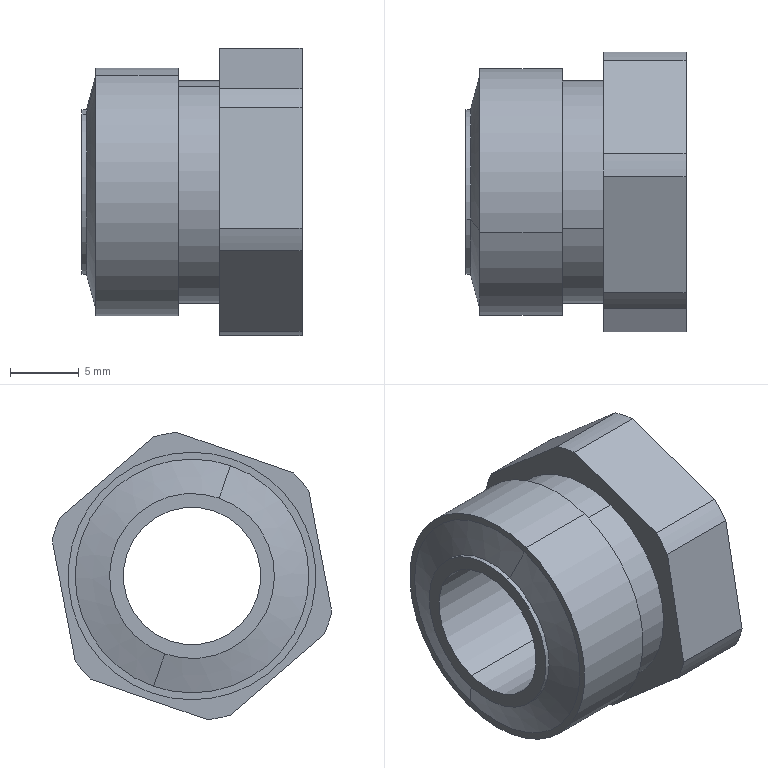Part | SolidWorks | features BaseBody 1 | 1 solid | 30 faces | box 16 x 20.336 x 20.886 mm | volume 2470 mm3 | cylinder 16 | plane 12 | cone 2 | commonest cylinder face diameters 21 x6 10 x2 12 x2 16 x2 16.2 x2 18 x2
STEP:
#1=CARTESIAN_POINT('',(0.03712,-55.457,-220.271));
#2=VERTEX_POINT('',#1);
#3=CARTESIAN_POINT('',(0.03712,-58.751,-210.829));
#4=VERTEX_POINT('',#3);
#5=CARTESIAN_POINT('',(0.03712,-57.104,-215.55));
#6=DIRECTION('',(-1.,0.,0.));
#7=DIRECTION('',(0.,0.3294,-0.9442));
#8=AXIS2_PLACEMENT_3D('',#5,#6,#7);
#9=CIRCLE('',#8,5.);
#10=EDGE_CURVE('',#2,#4,#9,.T.);
#11=ORIENTED_EDGE('',*,*,#10,.F.);
#12=CARTESIAN_POINT('',(-12.463,-55.457,-220.271));
#13=VERTEX_POINT('',#12);
#14=CARTESIAN_POINT('',(3.537,-55.457,-220.271));
#15=DIRECTION('',(-1.,0.,0.));
#16=VECTOR('',#15,1000.);
#17=LINE('',#14,#16);
#18=EDGE_CURVE('',#2,#13,#17,.T.);
#19=ORIENTED_EDGE('',*,*,#18,.T.);
#20=CARTESIAN_POINT('',(-12.463,-58.751,-210.829));
#21=VERTEX_POINT('',#20);
#22=CARTESIAN_POINT('',(-12.463,-57.104,-215.55));
#23=DIRECTION('',(-1.,0.,0.));
#24=DIRECTION('',(0.,-0.3294,0.9442));
#25=AXIS2_PLACEMENT_3D('',#22,#23,#24);
#26=CIRCLE('',#25,5.);
#27=EDGE_CURVE('',#13,#21,#26,.T.);
#28=ORIENTED_EDGE('',*,*,#27,.T.);
#29=CARTESIAN_POINT('',(3.537,-58.751,-210.829));
#30=DIRECTION('',(-1.,0.,0.));
#31=VECTOR('',#30,1000.);
#32=LINE('',#29,#31);
#33=EDGE_CURVE('',#4,#21,#32,.T.);
#34=ORIENTED_EDGE('',*,*,#33,.F.);
#35=EDGE_LOOP('',(#11,#19,#28,#34));
#36=FACE_OUTER_BOUND('',#35,.T.);
#37=CARTESIAN_POINT('',(3.537,-57.104,-215.55));
#38=DIRECTION('',(-1.,0.,0.));
#39=DIRECTION('',(0.,-0.3294,0.9442));
#40=AXIS2_PLACEMENT_3D('',#37,#38,#39);
#41=CYLINDRICAL_SURFACE('',#40,5.);
#42=ADVANCED_FACE('',(#36),#41,.F.);
#43=CARTESIAN_POINT('',(-5.463,-59.772,-207.902));
#44=VERTEX_POINT('',#43);
#45=CARTESIAN_POINT('',(-5.463,-54.435,-223.198));
#46=VERTEX_POINT('',#45);
#47=CARTESIAN_POINT('',(-5.463,-57.104,-215.55));
#48=DIRECTION('',(-1.,0.,0.));
#49=DIRECTION('',(0.,-0.3294,0.9442));
#50=AXIS2_PLACEMENT_3D('',#47,#48,#49);
#51=CIRCLE('',#50,8.1);
#52=EDGE_CURVE('',#44,#46,#51,.T.);
#53=ORIENTED_EDGE('',*,*,#52,.F.);
#54=CARTESIAN_POINT('',(-2.463,-59.772,-207.902));
#55=VERTEX_POINT('',#54);
#56=CARTESIAN_POINT('',(-5.463,-59.772,-207.902));
#57=DIRECTION('',(1.,0.,0.));
#58=VECTOR('',#57,1000.);
#59=LINE('',#56,#58);
#60=EDGE_CURVE('',#44,#55,#59,.T.);
#61=ORIENTED_EDGE('',*,*,#60,.T.);
#62=CARTESIAN_POINT('',(-2.463,-54.435,-223.198));
#63=VERTEX_POINT('',#62);
#64=CARTESIAN_POINT('',(-2.463,-57.104,-215.55));
#65=DIRECTION('',(-1.,0.,0.));
#66=DIRECTION('',(0.,-0.3294,0.9442));
#67=AXIS2_PLACEMENT_3D('',#64,#65,#66);
#68=CIRCLE('',#67,8.1);
#69=EDGE_CURVE('',#55,#63,#68,.T.);
#70=ORIENTED_EDGE('',*,*,#69,.T.);
#71=CARTESIAN_POINT('',(-5.463,-54.435,-223.198));
#72=DIRECTION('',(1.,0.,0.));
#73=VECTOR('',#72,1000.);
#74=LINE('',#71,#73);
#75=EDGE_CURVE('',#46,#63,#74,.T.);
#76=ORIENTED_EDGE('',*,*,#75,.F.);
#77=EDGE_LOOP('',(#53,#61,#70,#76));
#78=FACE_OUTER_BOUND('',#77,.T.);
#79=CARTESIAN_POINT('',(-5.463,-57.104,-215.55));
#80=DIRECTION('',(1.,0.,0.));
#81=DIRECTION('',(0.,0.3294,-0.9442));
#82=AXIS2_PLACEMENT_3D('',#79,#80,#81);
#83=CYLINDRICAL_SURFACE('',#82,8.1);
#84=ADVANCED_FACE('',(#78),#83,.T.);
#85=CARTESIAN_POINT('',(-11.463,-60.069,-207.052));
#86=VERTEX_POINT('',#85);
#87=CARTESIAN_POINT('',(-11.463,-54.139,-224.048));
#88=VERTEX_POINT('',#87);
#89=CARTESIAN_POINT('',(-11.463,-57.104,-215.55));
#90=DIRECTION('',(-1.,0.,0.));
#91=DIRECTION('',(0.,-0.3294,0.9442));
#92=AXIS2_PLACEMENT_3D('',#89,#90,#91);
#93=CIRCLE('',#92,9.);
#94=EDGE_CURVE('',#86,#88,#93,.T.);
#95=ORIENTED_EDGE('',*,*,#94,.F.);
#96=CARTESIAN_POINT('',(-5.463,-60.069,-207.052));
#97=VERTEX_POINT('',#96);
#98=CARTESIAN_POINT('',(-11.463,-60.069,-207.052));
#99=DIRECTION('',(1.,0.,0.));
#100=VECTOR('',#99,1000.);
#101=LINE('',#98,#100);
#102=EDGE_CURVE('',#86,#97,#101,.T.);
#103=ORIENTED_EDGE('',*,*,#102,.T.);
#104=CARTESIAN_POINT('',(-5.463,-54.139,-224.048));
#105=VERTEX_POINT('',#104);
#106=CARTESIAN_POINT('',(-5.463,-57.104,-215.55));
#107=DIRECTION('',(-1.,0.,0.));
#108=DIRECTION('',(0.,-0.3294,0.9442));
#109=AXIS2_PLACEMENT_3D('',#106,#107,#108);
#110=CIRCLE('',#109,9.);
#111=EDGE_CURVE('',#97,#105,#110,.T.);
#112=ORIENTED_EDGE('',*,*,#111,.T.);
#113=CARTESIAN_POINT('',(-11.463,-54.139,-224.048));
#114=DIRECTION('',(1.,0.,0.));
#115=VECTOR('',#114,1000.);
#116=LINE('',#113,#115);
#117=EDGE_CURVE('',#88,#105,#116,.T.);
#118=ORIENTED_EDGE('',*,*,#117,.F.);
#119=EDGE_LOOP('',(#95,#103,#112,#118));
#120=FACE_OUTER_BOUND('',#119,.T.);
#121=CARTESIAN_POINT('',(-11.463,-57.104,-215.55));
#122=DIRECTION('',(1.,0.,0.));
#123=DIRECTION('',(0.,0.3294,-0.9442));
#124=AXIS2_PLACEMENT_3D('',#121,#122,#123);
#125=CYLINDRICAL_SURFACE('',#124,9.);
#126=ADVANCED_FACE('',(#120),#125,.T.);
#127=CARTESIAN_POINT('',(-12.463,-59.08,-209.885));
#128=VERTEX_POINT('',#127);
#129=CARTESIAN_POINT('',(-12.463,-55.127,-221.215));
#130=VERTEX_POINT('',#129);
#131=CARTESIAN_POINT('',(-12.463,-57.104,-215.55));
#132=DIRECTION('',(-1.,0.,0.));
#133=DIRECTION('',(0.,-0.3294,0.9442));
#134=AXIS2_PLACEMENT_3D('',#131,#132,#133);
#135=CIRCLE('',#134,6.);
#136=EDGE_CURVE('',#128,#130,#135,.T.);
#137=ORIENTED_EDGE('',*,*,#136,.F.);
#138=CARTESIAN_POINT('',(-12.133,-59.08,-209.885));
#139=VERTEX_POINT('',#138);
#140=CARTESIAN_POINT('',(-12.463,-59.08,-209.885));
#141=DIRECTION('',(1.,0.,0.));
#142=VECTOR('',#141,1000.);
#143=LINE('',#140,#142);
#144=EDGE_CURVE('',#128,#139,#143,.T.);
#145=ORIENTED_EDGE('',*,*,#144,.T.);
#146=CARTESIAN_POINT('',(-12.133,-55.127,-221.215));
#147=VERTEX_POINT('',#146);
#148=CARTESIAN_POINT('',(-12.133,-57.104,-215.55));
#149=DIRECTION('',(-1.,0.,0.));
#150=DIRECTION('',(0.,-0.3294,0.9442));
#151=AXIS2_PLACEMENT_3D('',#148,#149,#150);
#152=CIRCLE('',#151,6.);
#153=EDGE_CURVE('',#139,#147,#152,.T.);
#154=ORIENTED_EDGE('',*,*,#153,.T.);
#155=CARTESIAN_POINT('',(-12.463,-55.127,-221.215));
#156=DIRECTION('',(1.,0.,0.));
#157=VECTOR('',#156,1000.);
#158=LINE('',#155,#157);
#159=EDGE_CURVE('',#130,#147,#158,.T.);
#160=ORIENTED_EDGE('',*,*,#159,.F.);
#161=EDGE_LOOP('',(#137,#145,#154,#160));
#162=FACE_OUTER_BOUND('',#161,.T.);
#163=CARTESIAN_POINT('',(-12.463,-57.104,-215.55));
#164=DIRECTION('',(1.,0.,0.));
#165=DIRECTION('',(0.,0.3294,-0.9442));
#166=AXIS2_PLACEMENT_3D('',#163,#164,#165);
#167=CYLINDRICAL_SURFACE('',#166,6.);
#168=ADVANCED_FACE('',(#162),#167,.T.);
#169=ORIENTED_EDGE('',*,*,#153,.F.);
#170=CARTESIAN_POINT('',(-11.463,-59.904,-207.525));
#171=VERTEX_POINT('',#170);
#172=CARTESIAN_POINT('',(-12.133,-59.08,-209.885));
#173=DIRECTION('',(0.2588,-0.3182,0.912));
#174=VECTOR('',#173,1000.);
#175=LINE('',#172,#174);
#176=EDGE_CURVE('',#139,#171,#175,.T.);
#177=ORIENTED_EDGE('',*,*,#176,.T.);
#178=CARTESIAN_POINT('',(-11.463,-54.303,-223.575));
#179=VERTEX_POINT('',#178);
#180=CARTESIAN_POINT('',(-11.463,-57.104,-215.55));
#181=DIRECTION('',(1.,0.,0.));
#182=DIRECTION('',(0.,-0.3294,0.9442));
#183=AXIS2_PLACEMENT_3D('',#180,#181,#182);
#184=CIRCLE('',#183,8.5);
#185=EDGE_CURVE('',#179,#171,#184,.T.);
#186=ORIENTED_EDGE('',*,*,#185,.F.);
#187=CARTESIAN_POINT('',(-12.133,-55.127,-221.215));
#188=DIRECTION('',(0.2588,0.3182,-0.912));
#189=VECTOR('',#188,1000.);
#190=LINE('',#187,#189);
#191=EDGE_CURVE('',#147,#179,#190,.T.);
#192=ORIENTED_EDGE('',*,*,#191,.F.);
#193=EDGE_LOOP('',(#169,#177,#186,#192));
#194=FACE_OUTER_BOUND('',#193,.T.);
#195=CARTESIAN_POINT('',(-12.133,-57.104,-215.55));
#196=DIRECTION('',(1.,0.,0.));
#197=DIRECTION('',(0.,0.3294,-0.9442));
#198=AXIS2_PLACEMENT_3D('',#195,#196,#197);
#199=CONICAL_SURFACE('',#198,6.,1.309);
#200=ADVANCED_FACE('',(#194),#199,.T.);
#201=CARTESIAN_POINT('',(0.03712,-59.739,-207.997));
#202=VERTEX_POINT('',#201);
#203=CARTESIAN_POINT('',(0.03712,-54.468,-223.103));
#204=VERTEX_POINT('',#203);
#205=CARTESIAN_POINT('',(0.03712,-57.104,-215.55));
#206=DIRECTION('',(1.,0.,0.));
#207=DIRECTION('',(0.,0.3294,-0.9442));
#208=AXIS2_PLACEMENT_3D('',#205,#206,#207);
#209=CIRCLE('',#208,8.);
#210=EDGE_CURVE('',#202,#204,#209,.T.);
#211=ORIENTED_EDGE('',*,*,#210,.F.);
#212=CARTESIAN_POINT('',(3.537,-59.739,-207.997));
#213=VERTEX_POINT('',#212);
#214=CARTESIAN_POINT('',(0.03712,-59.739,-207.997));
#215=DIRECTION('',(1.,0.,0.));
#216=VECTOR('',#215,1000.);
#217=LINE('',#214,#216);
#218=EDGE_CURVE('',#202,#213,#217,.T.);
#219=ORIENTED_EDGE('',*,*,#218,.T.);
#220=CARTESIAN_POINT('',(3.537,-54.468,-223.103));
#221=VERTEX_POINT('',#220);
#222=CARTESIAN_POINT('',(3.537,-57.104,-215.55));
#223=DIRECTION('',(1.,0.,0.));
#224=DIRECTION('',(0.,0.3294,-0.9442));
#225=AXIS2_PLACEMENT_3D('',#222,#223,#224);
#226=CIRCLE('',#225,8.);
#227=EDGE_CURVE('',#213,#221,#226,.T.);
#228=ORIENTED_EDGE('',*,*,#227,.T.);
#229=CARTESIAN_POINT('',(0.03712,-54.468,-223.103));
#230=DIRECTION('',(1.,0.,0.));
#231=VECTOR('',#230,1000.);
#232=LINE('',#229,#231);
#233=EDGE_CURVE('',#204,#221,#232,.T.);
#234=ORIENTED_EDGE('',*,*,#233,.F.);
#235=EDGE_LOOP('',(#211,#219,#228,#234));
#236=FACE_OUTER_BOUND('',#235,.T.);
#237=CARTESIAN_POINT('',(0.03712,-57.104,-215.55));
#238=DIRECTION('',(1.,0.,0.));
#239=DIRECTION('',(0.,0.3294,-0.9442));
#240=AXIS2_PLACEMENT_3D('',#237,#238,#239);
#241=CYLINDRICAL_SURFACE('',#240,8.);
#242=ADVANCED_FACE('',(#236),#241,.F.);
#243=CARTESIAN_POINT('',(-2.463,-65.601,-209.382));
#244=VERTEX_POINT('',#243);
#245=CARTESIAN_POINT('',(3.537,-65.601,-209.382));
#246=VERTEX_POINT('',#245);
#247=CARTESIAN_POINT('',(-2.463,-65.601,-209.382));
#248=DIRECTION('',(1.,0.,0.));
#249=VECTOR('',#248,1000.);
#250=LINE('',#247,#249);
#251=EDGE_CURVE('',#244,#246,#250,.T.);
#252=ORIENTED_EDGE('',*,*,#251,.F.);
#253=CARTESIAN_POINT('',(-2.463,-67.272,-218.169));
#254=VERTEX_POINT('',#253);
#255=CARTESIAN_POINT('',(-2.463,-66.437,-213.776));
#256=DIRECTION('',(0.,-0.1868,-0.9824));
#257=VECTOR('',#256,1000.);
#258=LINE('',#255,#257);
#259=EDGE_CURVE('',#244,#254,#258,.T.);
#260=ORIENTED_EDGE('',*,*,#259,.T.);
#261=CARTESIAN_POINT('',(3.537,-67.272,-218.169));
#262=VERTEX_POINT('',#261);
#263=CARTESIAN_POINT('',(-2.463,-67.272,-218.169));
#264=DIRECTION('',(-1.,0.,0.));
#265=VECTOR('',#264,1000.);
#266=LINE('',#263,#265);
#267=EDGE_CURVE('',#262,#254,#266,.T.);
#268=ORIENTED_EDGE('',*,*,#267,.F.);
#269=CARTESIAN_POINT('',(3.537,-67.461,-219.164));
#270=DIRECTION('',(0.,0.1868,0.9824));
#271=VECTOR('',#270,1000.);
#272=LINE('',#269,#271);
#273=EDGE_CURVE('',#262,#246,#272,.T.);
#274=ORIENTED_EDGE('',*,*,#273,.T.);
#275=EDGE_LOOP('',(#252,#260,#268,#274));
#276=FACE_OUTER_BOUND('',#275,.T.);
#277=CARTESIAN_POINT('',(-12.463,-67.461,-219.164));
#278=DIRECTION('',(0.,0.9824,-0.1868));
#279=DIRECTION('',(-1.,0.,0.));
#280=AXIS2_PLACEMENT_3D('',#277,#278,#279);
#281=PLANE('',#280);
#282=ADVANCED_FACE('',(#276),#281,.F.);
#283=CARTESIAN_POINT('',(-2.463,-64.456,-208.054));
#284=VERTEX_POINT('',#283);
#285=CARTESIAN_POINT('',(-2.463,-56.011,-205.107));
#286=VERTEX_POINT('',#285);
#287=CARTESIAN_POINT('',(-2.463,-60.234,-206.58));
#288=DIRECTION('',(0.,0.9442,0.3294));
#289=VECTOR('',#288,1000.);
#290=LINE('',#287,#289);
#291=EDGE_CURVE('',#284,#286,#290,.T.);
#292=ORIENTED_EDGE('',*,*,#291,.F.);
#293=CARTESIAN_POINT('',(3.537,-64.456,-208.054));
#294=VERTEX_POINT('',#293);
#295=CARTESIAN_POINT('',(-2.463,-64.456,-208.054));
#296=DIRECTION('',(1.,0.,0.));
#297=VECTOR('',#296,1000.);
#298=LINE('',#295,#297);
#299=EDGE_CURVE('',#284,#294,#298,.T.);
#300=ORIENTED_EDGE('',*,*,#299,.T.);
#301=CARTESIAN_POINT('',(3.537,-56.011,-205.107));
#302=VERTEX_POINT('',#301);
#303=CARTESIAN_POINT('',(3.537,-55.055,-204.773));
#304=DIRECTION('',(0.,-0.9442,-0.3294));
#305=VECTOR('',#304,1000.);
#306=LINE('',#303,#305);
#307=EDGE_CURVE('',#302,#294,#306,.T.);
#308=ORIENTED_EDGE('',*,*,#307,.F.);
#309=CARTESIAN_POINT('',(-2.463,-56.011,-205.107));
#310=DIRECTION('',(-1.,0.,0.));
#311=VECTOR('',#310,1000.);
#312=LINE('',#309,#311);
#313=EDGE_CURVE('',#302,#286,#312,.T.);
#314=ORIENTED_EDGE('',*,*,#313,.T.);
#315=EDGE_LOOP('',(#292,#300,#308,#314));
#316=FACE_OUTER_BOUND('',#315,.T.);
#317=CARTESIAN_POINT('',(-12.463,-55.055,-204.773));
#318=DIRECTION('',(0.,-0.3294,0.9442));
#319=DIRECTION('',(-1.,0.,0.));
#320=AXIS2_PLACEMENT_3D('',#317,#318,#319);
#321=PLANE('',#320);
#322=ADVANCED_FACE('',(#316),#321,.T.);
#323=CARTESIAN_POINT('',(-2.463,-54.288,-205.435));
#324=VERTEX_POINT('',#323);
#325=CARTESIAN_POINT('',(-2.463,-47.514,-211.275));
#326=VERTEX_POINT('',#325);
#327=CARTESIAN_POINT('',(-2.463,-50.901,-208.355));
#328=DIRECTION('',(0.,0.7574,-0.653));
#329=VECTOR('',#328,1000.);
#330=LINE('',#327,#329);
#331=EDGE_CURVE('',#324,#326,#330,.T.);
#332=ORIENTED_EDGE('',*,*,#331,.F.);
#333=CARTESIAN_POINT('',(3.537,-54.288,-205.435));
#334=VERTEX_POINT('',#333);
#335=CARTESIAN_POINT('',(-2.463,-54.288,-205.435));
#336=DIRECTION('',(1.,0.,0.));
#337=VECTOR('',#336,1000.);
#338=LINE('',#335,#337);
#339=EDGE_CURVE('',#324,#334,#338,.T.);
#340=ORIENTED_EDGE('',*,*,#339,.T.);
#341=CARTESIAN_POINT('',(3.537,-47.514,-211.275));
#342=VERTEX_POINT('',#341);
#343=CARTESIAN_POINT('',(3.537,-46.747,-211.936));
#344=DIRECTION('',(0.,-0.7574,0.653));
#345=VECTOR('',#344,1000.);
#346=LINE('',#343,#345);
#347=EDGE_CURVE('',#342,#334,#346,.T.);
#348=ORIENTED_EDGE('',*,*,#347,.F.);
#349=CARTESIAN_POINT('',(-2.463,-47.514,-211.275));
#350=DIRECTION('',(-1.,0.,0.));
#351=VECTOR('',#350,1000.);
#352=LINE('',#349,#351);
#353=EDGE_CURVE('',#342,#326,#352,.T.);
#354=ORIENTED_EDGE('',*,*,#353,.T.);
#355=EDGE_LOOP('',(#332,#340,#348,#354));
#356=FACE_OUTER_BOUND('',#355,.T.);
#357=CARTESIAN_POINT('',(-12.463,-46.747,-211.936));
#358=DIRECTION('',(0.,0.653,0.7574));
#359=DIRECTION('',(1.,0.,0.));
#360=AXIS2_PLACEMENT_3D('',#357,#358,#359);
#361=PLANE('',#360);
#362=ADVANCED_FACE('',(#356),#361,.T.);
#363=CARTESIAN_POINT('',(-2.463,-48.606,-221.718));
#364=VERTEX_POINT('',#363);
#365=CARTESIAN_POINT('',(3.537,-48.606,-221.718));
#366=VERTEX_POINT('',#365);
#367=CARTESIAN_POINT('',(-2.463,-48.606,-221.718));
#368=DIRECTION('',(1.,0.,0.));
#369=VECTOR('',#368,1000.);
#370=LINE('',#367,#369);
#371=EDGE_CURVE('',#364,#366,#370,.T.);
#372=ORIENTED_EDGE('',*,*,#371,.F.);
#373=CARTESIAN_POINT('',(-2.463,-46.936,-212.931));
#374=VERTEX_POINT('',#373);
#375=CARTESIAN_POINT('',(-2.463,-47.771,-217.324));
#376=DIRECTION('',(0.,0.1868,0.9824));
#377=VECTOR('',#376,1000.);
#378=LINE('',#375,#377);
#379=EDGE_CURVE('',#364,#374,#378,.T.);
#380=ORIENTED_EDGE('',*,*,#379,.T.);
#381=CARTESIAN_POINT('',(3.537,-46.936,-212.931));
#382=VERTEX_POINT('',#381);
#383=CARTESIAN_POINT('',(-2.463,-46.936,-212.931));
#384=DIRECTION('',(-1.,0.,0.));
#385=VECTOR('',#384,1000.);
#386=LINE('',#383,#385);
#387=EDGE_CURVE('',#382,#374,#386,.T.);
#388=ORIENTED_EDGE('',*,*,#387,.F.);
#389=CARTESIAN_POINT('',(3.537,-46.747,-211.936));
#390=DIRECTION('',(0.,-0.1868,-0.9824));
#391=VECTOR('',#390,1000.);
#392=LINE('',#389,#391);
#393=EDGE_CURVE('',#382,#366,#392,.T.);
#394=ORIENTED_EDGE('',*,*,#393,.T.);
#395=EDGE_LOOP('',(#372,#380,#388,#394));
#396=FACE_OUTER_BOUND('',#395,.T.);
#397=CARTESIAN_POINT('',(-12.463,-46.747,-211.936));
#398=DIRECTION('',(0.,-0.9824,0.1868));
#399=DIRECTION('',(-1.,0.,0.));
#400=AXIS2_PLACEMENT_3D('',#397,#398,#399);
#401=PLANE('',#400);
#402=ADVANCED_FACE('',(#396),#401,.F.);
#403=CARTESIAN_POINT('',(-2.463,-58.196,-225.993));
#404=VERTEX_POINT('',#403);
#405=CARTESIAN_POINT('',(3.537,-58.196,-225.993));
#406=VERTEX_POINT('',#405);
#407=CARTESIAN_POINT('',(-2.463,-58.196,-225.993));
#408=DIRECTION('',(1.,0.,0.));
#409=VECTOR('',#408,1000.);
#410=LINE('',#407,#409);
#411=EDGE_CURVE('',#404,#406,#410,.T.);
#412=ORIENTED_EDGE('',*,*,#411,.F.);
#413=CARTESIAN_POINT('',(-2.463,-49.752,-223.046));
#414=VERTEX_POINT('',#413);
#415=CARTESIAN_POINT('',(-2.463,-53.974,-224.52));
#416=DIRECTION('',(0.,0.9442,0.3294));
#417=VECTOR('',#416,1000.);
#418=LINE('',#415,#417);
#419=EDGE_CURVE('',#404,#414,#418,.T.);
#420=ORIENTED_EDGE('',*,*,#419,.T.);
#421=CARTESIAN_POINT('',(3.537,-49.752,-223.046));
#422=VERTEX_POINT('',#421);
#423=CARTESIAN_POINT('',(-2.463,-49.752,-223.046));
#424=DIRECTION('',(-1.,0.,0.));
#425=VECTOR('',#424,1000.);
#426=LINE('',#423,#425);
#427=EDGE_CURVE('',#422,#414,#426,.T.);
#428=ORIENTED_EDGE('',*,*,#427,.F.);
#429=CARTESIAN_POINT('',(3.537,-48.795,-222.713));
#430=DIRECTION('',(0.,-0.9442,-0.3294));
#431=VECTOR('',#430,1000.);
#432=LINE('',#429,#431);
#433=EDGE_CURVE('',#422,#406,#432,.T.);
#434=ORIENTED_EDGE('',*,*,#433,.T.);
#435=EDGE_LOOP('',(#412,#420,#428,#434));
#436=FACE_OUTER_BOUND('',#435,.T.);
#437=CARTESIAN_POINT('',(-12.463,-48.795,-222.713));
#438=DIRECTION('',(0.,-0.3294,0.9442));
#439=DIRECTION('',(-1.,0.,0.));
#440=AXIS2_PLACEMENT_3D('',#437,#438,#439);
#441=PLANE('',#440);
#442=ADVANCED_FACE('',(#436),#441,.F.);
#443=CARTESIAN_POINT('',(-2.463,-59.92,-225.665));
#444=VERTEX_POINT('',#443);
#445=CARTESIAN_POINT('',(-2.463,-66.694,-219.825));
#446=VERTEX_POINT('',#445);
#447=CARTESIAN_POINT('',(-2.463,-63.307,-222.745));
#448=DIRECTION('',(0.,-0.7574,0.653));
#449=VECTOR('',#448,1000.);
#450=LINE('',#447,#449);
#451=EDGE_CURVE('',#444,#446,#450,.T.);
#452=ORIENTED_EDGE('',*,*,#451,.F.);
#453=CARTESIAN_POINT('',(3.537,-59.92,-225.665));
#454=VERTEX_POINT('',#453);
#455=CARTESIAN_POINT('',(-2.463,-59.92,-225.665));
#456=DIRECTION('',(1.,0.,0.));
#457=VECTOR('',#456,1000.);
#458=LINE('',#455,#457);
#459=EDGE_CURVE('',#444,#454,#458,.T.);
#460=ORIENTED_EDGE('',*,*,#459,.T.);
#461=CARTESIAN_POINT('',(3.537,-66.694,-219.825));
#462=VERTEX_POINT('',#461);
#463=CARTESIAN_POINT('',(3.537,-67.461,-219.164));
#464=DIRECTION('',(0.,0.7574,-0.653));
#465=VECTOR('',#464,1000.);
#466=LINE('',#463,#465);
#467=EDGE_CURVE('',#462,#454,#466,.T.);
#468=ORIENTED_EDGE('',*,*,#467,.F.);
#469=CARTESIAN_POINT('',(-2.463,-66.694,-219.825));
#470=DIRECTION('',(-1.,0.,0.));
#471=VECTOR('',#470,1000.);
#472=LINE('',#469,#471);
#473=EDGE_CURVE('',#462,#446,#472,.T.);
#474=ORIENTED_EDGE('',*,*,#473,.T.);
#475=EDGE_LOOP('',(#452,#460,#468,#474));
#476=FACE_OUTER_BOUND('',#475,.T.);
#477=CARTESIAN_POINT('',(-12.463,-67.461,-219.164));
#478=DIRECTION('',(0.,-0.653,-0.7574));
#479=DIRECTION('',(0.,-0.7574,0.653));
#480=AXIS2_PLACEMENT_3D('',#477,#478,#479);
#481=PLANE('',#480);
#482=ADVANCED_FACE('',(#476),#481,.T.);
#483=ORIENTED_EDGE('',*,*,#218,.F.);
#484=CARTESIAN_POINT('',(0.03712,-57.104,-215.55));
#485=DIRECTION('',(1.,0.,0.));
#486=DIRECTION('',(0.,0.3294,-0.9442));
#487=AXIS2_PLACEMENT_3D('',#484,#485,#486);
#488=CIRCLE('',#487,8.);
#489=EDGE_CURVE('',#204,#202,#488,.T.);
#490=ORIENTED_EDGE('',*,*,#489,.F.);
#491=ORIENTED_EDGE('',*,*,#233,.T.);
#492=CARTESIAN_POINT('',(3.537,-57.104,-215.55));
#493=DIRECTION('',(1.,0.,0.));
#494=DIRECTION('',(0.,0.3294,-0.9442));
#495=AXIS2_PLACEMENT_3D('',#492,#493,#494);
#496=CIRCLE('',#495,8.);
#497=EDGE_CURVE('',#221,#213,#496,.T.);
#498=ORIENTED_EDGE('',*,*,#497,.T.);
#499=EDGE_LOOP('',(#483,#490,#491,#498));
#500=FACE_OUTER_BOUND('',#499,.T.);
#501=CARTESIAN_POINT('',(0.03712,-57.104,-215.55));
#502=DIRECTION('',(1.,0.,0.));
#503=DIRECTION('',(0.,0.3294,-0.9442));
#504=AXIS2_PLACEMENT_3D('',#501,#502,#503);
#505=CYLINDRICAL_SURFACE('',#504,8.);
#506=ADVANCED_FACE('',(#500),#505,.F.);
#507=CARTESIAN_POINT('',(0.03712,-57.104,-215.55));
#508=DIRECTION('',(-1.,0.,0.));
#509=DIRECTION('',(0.,0.3294,-0.9442));
#510=AXIS2_PLACEMENT_3D('',#507,#508,#509);
#511=CIRCLE('',#510,5.);
#512=EDGE_CURVE('',#4,#2,#511,.T.);
#513=ORIENTED_EDGE('',*,*,#512,.T.);
#514=ORIENTED_EDGE('',*,*,#10,.T.);
#515=EDGE_LOOP('',(#513,#514));
#516=FACE_BOUND('',#515,.T.);
#517=ORIENTED_EDGE('',*,*,#489,.T.);
#518=ORIENTED_EDGE('',*,*,#210,.T.);
#519=EDGE_LOOP('',(#517,#518));
#520=FACE_OUTER_BOUND('',#519,.T.);
#521=CARTESIAN_POINT('',(0.03712,-57.104,-215.55));
#522=DIRECTION('',(1.,0.,0.));
#523=DIRECTION('',(0.,0.,-1.));
#524=AXIS2_PLACEMENT_3D('',#521,#522,#523);
#525=PLANE('',#524);
#526=ADVANCED_FACE('',(#516,#520),#525,.T.);
#527=ORIENTED_EDGE('',*,*,#176,.F.);
#528=CARTESIAN_POINT('',(-12.133,-57.104,-215.55));
#529=DIRECTION('',(-1.,0.,0.));
#530=DIRECTION('',(0.,-0.3294,0.9442));
#531=AXIS2_PLACEMENT_3D('',#528,#529,#530);
#532=CIRCLE('',#531,6.);
#533=EDGE_CURVE('',#147,#139,#532,.T.);
#534=ORIENTED_EDGE('',*,*,#533,.F.);
#535=ORIENTED_EDGE('',*,*,#191,.T.);
#536=CARTESIAN_POINT('',(-11.463,-57.104,-215.55));
#537=DIRECTION('',(1.,0.,0.));
#538=DIRECTION('',(0.,-0.3294,0.9442));
#539=AXIS2_PLACEMENT_3D('',#536,#537,#538);
#540=CIRCLE('',#539,8.5);
#541=EDGE_CURVE('',#171,#179,#540,.T.);
#542=ORIENTED_EDGE('',*,*,#541,.F.);
#543=EDGE_LOOP('',(#527,#534,#535,#542));
#544=FACE_OUTER_BOUND('',#543,.T.);
#545=CARTESIAN_POINT('',(-12.133,-57.104,-215.55));
#546=DIRECTION('',(1.,0.,0.));
#547=DIRECTION('',(0.,0.3294,-0.9442));
#548=AXIS2_PLACEMENT_3D('',#545,#546,#547);
#549=CONICAL_SURFACE('',#548,6.,1.309);
#550=ADVANCED_FACE('',(#544),#549,.T.);
#551=CARTESIAN_POINT('',(-12.463,-57.104,-215.55));
#552=DIRECTION('',(-1.,0.,0.));
#553=DIRECTION('',(0.,-0.3294,0.9442));
#554=AXIS2_PLACEMENT_3D('',#551,#552,#553);
#555=CIRCLE('',#554,6.);
#556=EDGE_CURVE('',#130,#128,#555,.T.);
#557=ORIENTED_EDGE('',*,*,#556,.T.);
#558=ORIENTED_EDGE('',*,*,#136,.T.);
#559=EDGE_LOOP('',(#557,#558));
#560=FACE_OUTER_BOUND('',#559,.T.);
#561=CARTESIAN_POINT('',(-12.463,-57.104,-215.55));
#562=DIRECTION('',(-1.,0.,0.));
#563=DIRECTION('',(0.,-0.3294,0.9442));
#564=AXIS2_PLACEMENT_3D('',#561,#562,#563);
#565=CIRCLE('',#564,5.);
#566=EDGE_CURVE('',#21,#13,#565,.T.);
#567=ORIENTED_EDGE('',*,*,#566,.F.);
#568=ORIENTED_EDGE('',*,*,#27,.F.);
#569=EDGE_LOOP('',(#567,#568));
#570=FACE_BOUND('',#569,.T.);
#571=CARTESIAN_POINT('',(-12.463,-57.104,-215.55));
#572=DIRECTION('',(-1.,0.,0.));
#573=DIRECTION('',(0.,1.,0.));
#574=AXIS2_PLACEMENT_3D('',#571,#572,#573);
#575=PLANE('',#574);
#576=ADVANCED_FACE('',(#560,#570),#575,.T.);
#577=ORIENTED_EDGE('',*,*,#144,.F.);
#578=ORIENTED_EDGE('',*,*,#556,.F.);
#579=ORIENTED_EDGE('',*,*,#159,.T.);
#580=ORIENTED_EDGE('',*,*,#533,.T.);
#581=EDGE_LOOP('',(#577,#578,#579,#580));
#582=FACE_OUTER_BOUND('',#581,.T.);
#583=CARTESIAN_POINT('',(-12.463,-57.104,-215.55));
#584=DIRECTION('',(1.,0.,0.));
#585=DIRECTION('',(0.,0.3294,-0.9442));
#586=AXIS2_PLACEMENT_3D('',#583,#584,#585);
#587=CYLINDRICAL_SURFACE('',#586,6.);
#588=ADVANCED_FACE('',(#582),#587,.T.);
#589=ORIENTED_EDGE('',*,*,#102,.F.);
#590=CARTESIAN_POINT('',(-11.463,-57.104,-215.55));
#591=DIRECTION('',(-1.,0.,0.));
#592=DIRECTION('',(0.,-0.3294,0.9442));
#593=AXIS2_PLACEMENT_3D('',#590,#591,#592);
#594=CIRCLE('',#593,9.);
#595=EDGE_CURVE('',#88,#86,#594,.T.);
#596=ORIENTED_EDGE('',*,*,#595,.F.);
#597=ORIENTED_EDGE('',*,*,#117,.T.);
#598=CARTESIAN_POINT('',(-5.463,-57.104,-215.55));
#599=DIRECTION('',(-1.,0.,0.));
#600=DIRECTION('',(0.,-0.3294,0.9442));
#601=AXIS2_PLACEMENT_3D('',#598,#599,#600);
#602=CIRCLE('',#601,9.);
#603=EDGE_CURVE('',#105,#97,#602,.T.);
#604=ORIENTED_EDGE('',*,*,#603,.T.);
#605=EDGE_LOOP('',(#589,#596,#597,#604));
#606=FACE_OUTER_BOUND('',#605,.T.);
#607=CARTESIAN_POINT('',(-11.463,-57.104,-215.55));
#608=DIRECTION('',(1.,0.,0.));
#609=DIRECTION('',(0.,0.3294,-0.9442));
#610=AXIS2_PLACEMENT_3D('',#607,#608,#609);
#611=CYLINDRICAL_SURFACE('',#610,9.);
#612=ADVANCED_FACE('',(#606),#611,.T.);
#613=CARTESIAN_POINT('',(-5.463,-57.104,-215.55));
#614=DIRECTION('',(-1.,0.,0.));
#615=DIRECTION('',(0.,-0.3294,0.9442));
#616=AXIS2_PLACEMENT_3D('',#613,#614,#615);
#617=CIRCLE('',#616,8.1);
#618=EDGE_CURVE('',#46,#44,#617,.T.);
#619=ORIENTED_EDGE('',*,*,#618,.T.);
#620=ORIENTED_EDGE('',*,*,#52,.T.);
#621=EDGE_LOOP('',(#619,#620));
#622=FACE_BOUND('',#621,.T.);
#623=ORIENTED_EDGE('',*,*,#603,.F.);
#624=ORIENTED_EDGE('',*,*,#111,.F.);
#625=EDGE_LOOP('',(#623,#624));
#626=FACE_OUTER_BOUND('',#625,.T.);
#627=CARTESIAN_POINT('',(-5.463,-57.104,-215.55));
#628=DIRECTION('',(-1.,0.,0.));
#629=DIRECTION('',(0.,1.,0.));
#630=AXIS2_PLACEMENT_3D('',#627,#628,#629);
#631=PLANE('',#630);
#632=ADVANCED_FACE('',(#622,#626),#631,.F.);
#633=ORIENTED_EDGE('',*,*,#60,.F.);
#634=ORIENTED_EDGE('',*,*,#618,.F.);
#635=ORIENTED_EDGE('',*,*,#75,.T.);
#636=CARTESIAN_POINT('',(-2.463,-57.104,-215.55));
#637=DIRECTION('',(-1.,0.,0.));
#638=DIRECTION('',(0.,-0.3294,0.9442));
#639=AXIS2_PLACEMENT_3D('',#636,#637,#638);
#640=CIRCLE('',#639,8.1);
#641=EDGE_CURVE('',#63,#55,#640,.T.);
#642=ORIENTED_EDGE('',*,*,#641,.T.);
#643=EDGE_LOOP('',(#633,#634,#635,#642));
#644=FACE_OUTER_BOUND('',#643,.T.);
#645=CARTESIAN_POINT('',(-5.463,-57.104,-215.55));
#646=DIRECTION('',(1.,0.,0.));
#647=DIRECTION('',(0.,0.3294,-0.9442));
#648=AXIS2_PLACEMENT_3D('',#645,#646,#647);
#649=CYLINDRICAL_SURFACE('',#648,8.1);
#650=ADVANCED_FACE('',(#644),#649,.T.);
#651=ORIENTED_EDGE('',*,*,#595,.T.);
#652=ORIENTED_EDGE('',*,*,#94,.T.);
#653=EDGE_LOOP('',(#651,#652));
#654=FACE_OUTER_BOUND('',#653,.T.);
#655=ORIENTED_EDGE('',*,*,#185,.T.);
#656=ORIENTED_EDGE('',*,*,#541,.T.);
#657=EDGE_LOOP('',(#655,#656));
#658=FACE_BOUND('',#657,.T.);
#659=CARTESIAN_POINT('',(-11.463,-57.104,-215.55));
#660=DIRECTION('',(-1.,0.,0.));
#661=DIRECTION('',(0.,1.,0.));
#662=AXIS2_PLACEMENT_3D('',#659,#660,#661);
#663=PLANE('',#662);
#664=ADVANCED_FACE('',(#654,#658),#663,.T.);
#665=ORIENTED_EDGE('',*,*,#18,.F.);
#666=ORIENTED_EDGE('',*,*,#512,.F.);
#667=ORIENTED_EDGE('',*,*,#33,.T.);
#668=ORIENTED_EDGE('',*,*,#566,.T.);
#669=EDGE_LOOP('',(#665,#666,#667,#668));
#670=FACE_OUTER_BOUND('',#669,.T.);
#671=CARTESIAN_POINT('',(3.537,-57.104,-215.55));
#672=DIRECTION('',(-1.,0.,0.));
#673=DIRECTION('',(0.,-0.3294,0.9442));
#674=AXIS2_PLACEMENT_3D('',#671,#672,#673);
#675=CYLINDRICAL_SURFACE('',#674,5.);
#676=ADVANCED_FACE('',(#670),#675,.F.);
#677=CARTESIAN_POINT('',(3.537,-57.104,-215.55));
#678=DIRECTION('',(-1.,0.,0.));
#679=DIRECTION('',(0.,-0.3294,0.9442));
#680=AXIS2_PLACEMENT_3D('',#677,#678,#679);
#681=CIRCLE('',#680,10.5);
#682=EDGE_CURVE('',#246,#294,#681,.T.);
#683=ORIENTED_EDGE('',*,*,#682,.F.);
#684=ORIENTED_EDGE('',*,*,#273,.F.);
#685=CARTESIAN_POINT('',(3.537,-57.104,-215.55));
#686=DIRECTION('',(-1.,0.,0.));
#687=DIRECTION('',(0.,-0.3294,0.9442));
#688=AXIS2_PLACEMENT_3D('',#685,#686,#687);
#689=CIRCLE('',#688,10.5);
#690=EDGE_CURVE('',#462,#262,#689,.T.);
#691=ORIENTED_EDGE('',*,*,#690,.F.);
#692=ORIENTED_EDGE('',*,*,#467,.T.);
#693=CARTESIAN_POINT('',(3.537,-57.104,-215.55));
#694=DIRECTION('',(-1.,0.,0.));
#695=DIRECTION('',(0.,-0.3294,0.9442));
#696=AXIS2_PLACEMENT_3D('',#693,#694,#695);
#697=CIRCLE('',#696,10.5);
#698=EDGE_CURVE('',#406,#454,#697,.T.);
#699=ORIENTED_EDGE('',*,*,#698,.F.);
#700=ORIENTED_EDGE('',*,*,#433,.F.);
#701=CARTESIAN_POINT('',(3.537,-57.104,-215.55));
#702=DIRECTION('',(-1.,0.,0.));
#703=DIRECTION('',(0.,-0.3294,0.9442));
#704=AXIS2_PLACEMENT_3D('',#701,#702,#703);
#705=CIRCLE('',#704,10.5);
#706=EDGE_CURVE('',#366,#422,#705,.T.);
#707=ORIENTED_EDGE('',*,*,#706,.F.);
#708=ORIENTED_EDGE('',*,*,#393,.F.);
#709=CARTESIAN_POINT('',(3.537,-57.104,-215.55));
#710=DIRECTION('',(-1.,0.,0.));
#711=DIRECTION('',(0.,-0.3294,0.9442));
#712=AXIS2_PLACEMENT_3D('',#709,#710,#711);
#713=CIRCLE('',#712,10.5);
#714=EDGE_CURVE('',#342,#382,#713,.T.);
#715=ORIENTED_EDGE('',*,*,#714,.F.);
#716=ORIENTED_EDGE('',*,*,#347,.T.);
#717=CARTESIAN_POINT('',(3.537,-57.104,-215.55));
#718=DIRECTION('',(-1.,0.,0.));
#719=DIRECTION('',(0.,-0.3294,0.9442));
#720=AXIS2_PLACEMENT_3D('',#717,#718,#719);
#721=CIRCLE('',#720,10.5);
#722=EDGE_CURVE('',#302,#334,#721,.T.);
#723=ORIENTED_EDGE('',*,*,#722,.F.);
#724=ORIENTED_EDGE('',*,*,#307,.T.);
#725=EDGE_LOOP('',(#683,#684,#691,#692,#699,#700,#707,#708,#715,#716,#723,#724));
#726=FACE_OUTER_BOUND('',#725,.T.);
#727=ORIENTED_EDGE('',*,*,#497,.F.);
#728=ORIENTED_EDGE('',*,*,#227,.F.);
#729=EDGE_LOOP('',(#727,#728));
#730=FACE_BOUND('',#729,.T.);
#731=CARTESIAN_POINT('',(3.537,-57.104,-215.55));
#732=DIRECTION('',(-1.,0.,0.));
#733=DIRECTION('',(0.,1.,0.));
#734=AXIS2_PLACEMENT_3D('',#731,#732,#733);
#735=PLANE('',#734);
#736=ADVANCED_FACE('',(#726,#730),#735,.F.);
#737=CARTESIAN_POINT('',(-2.463,-57.104,-215.55));
#738=DIRECTION('',(-1.,0.,0.));
#739=DIRECTION('',(0.,-0.3294,0.9442));
#740=AXIS2_PLACEMENT_3D('',#737,#738,#739);
#741=CIRCLE('',#740,10.5);
#742=EDGE_CURVE('',#404,#444,#741,.T.);
#743=ORIENTED_EDGE('',*,*,#742,.F.);
#744=ORIENTED_EDGE('',*,*,#411,.T.);
#745=ORIENTED_EDGE('',*,*,#698,.T.);
#746=ORIENTED_EDGE('',*,*,#459,.F.);
#747=EDGE_LOOP('',(#743,#744,#745,#746));
#748=FACE_OUTER_BOUND('',#747,.T.);
#749=CARTESIAN_POINT('',(-2.463,-57.104,-215.55));
#750=DIRECTION('',(1.,0.,0.));
#751=DIRECTION('',(0.,0.3294,-0.9442));
#752=AXIS2_PLACEMENT_3D('',#749,#750,#751);
#753=CYLINDRICAL_SURFACE('',#752,10.5);
#754=ADVANCED_FACE('',(#748),#753,.T.);
#755=ORIENTED_EDGE('',*,*,#353,.F.);
#756=ORIENTED_EDGE('',*,*,#714,.T.);
#757=ORIENTED_EDGE('',*,*,#387,.T.);
#758=CARTESIAN_POINT('',(-2.463,-57.104,-215.55));
#759=DIRECTION('',(-1.,0.,0.));
#760=DIRECTION('',(0.,-0.3294,0.9442));
#761=AXIS2_PLACEMENT_3D('',#758,#759,#760);
#762=CIRCLE('',#761,10.5);
#763=EDGE_CURVE('',#326,#374,#762,.T.);
#764=ORIENTED_EDGE('',*,*,#763,.F.);
#765=EDGE_LOOP('',(#755,#756,#757,#764));
#766=FACE_OUTER_BOUND('',#765,.T.);
#767=CARTESIAN_POINT('',(-2.463,-57.104,-215.55));
#768=DIRECTION('',(1.,0.,0.));
#769=DIRECTION('',(0.,0.3294,-0.9442));
#770=AXIS2_PLACEMENT_3D('',#767,#768,#769);
#771=CYLINDRICAL_SURFACE('',#770,10.5);
#772=ADVANCED_FACE('',(#766),#771,.T.);
#773=CARTESIAN_POINT('',(-2.463,-57.104,-215.55));
#774=DIRECTION('',(-1.,0.,0.));
#775=DIRECTION('',(0.,-0.3294,0.9442));
#776=AXIS2_PLACEMENT_3D('',#773,#774,#775);
#777=CIRCLE('',#776,10.5);
#778=EDGE_CURVE('',#364,#414,#777,.T.);
#779=ORIENTED_EDGE('',*,*,#778,.F.);
#780=ORIENTED_EDGE('',*,*,#371,.T.);
#781=ORIENTED_EDGE('',*,*,#706,.T.);
#782=ORIENTED_EDGE('',*,*,#427,.T.);
#783=EDGE_LOOP('',(#779,#780,#781,#782));
#784=FACE_OUTER_BOUND('',#783,.T.);
#785=CARTESIAN_POINT('',(-2.463,-57.104,-215.55));
#786=DIRECTION('',(1.,0.,0.));
#787=DIRECTION('',(0.,0.3294,-0.9442));
#788=AXIS2_PLACEMENT_3D('',#785,#786,#787);
#789=CYLINDRICAL_SURFACE('',#788,10.5);
#790=ADVANCED_FACE('',(#784),#789,.T.);
#791=ORIENTED_EDGE('',*,*,#313,.F.);
#792=ORIENTED_EDGE('',*,*,#722,.T.);
#793=ORIENTED_EDGE('',*,*,#339,.F.);
#794=CARTESIAN_POINT('',(-2.463,-57.104,-215.55));
#795=DIRECTION('',(-1.,0.,0.));
#796=DIRECTION('',(0.,-0.3294,0.9442));
#797=AXIS2_PLACEMENT_3D('',#794,#795,#796);
#798=CIRCLE('',#797,10.5);
#799=EDGE_CURVE('',#286,#324,#798,.T.);
#800=ORIENTED_EDGE('',*,*,#799,.F.);
#801=EDGE_LOOP('',(#791,#792,#793,#800));
#802=FACE_OUTER_BOUND('',#801,.T.);
#803=CARTESIAN_POINT('',(-2.463,-57.104,-215.55));
#804=DIRECTION('',(1.,0.,0.));
#805=DIRECTION('',(0.,0.3294,-0.9442));
#806=AXIS2_PLACEMENT_3D('',#803,#804,#805);
#807=CYLINDRICAL_SURFACE('',#806,10.5);
#808=ADVANCED_FACE('',(#802),#807,.T.);
#809=ORIENTED_EDGE('',*,*,#690,.T.);
#810=ORIENTED_EDGE('',*,*,#267,.T.);
#811=CARTESIAN_POINT('',(-2.463,-57.104,-215.55));
#812=DIRECTION('',(-1.,0.,0.));
#813=DIRECTION('',(0.,-0.3294,0.9442));
#814=AXIS2_PLACEMENT_3D('',#811,#812,#813);
#815=CIRCLE('',#814,10.5);
#816=EDGE_CURVE('',#446,#254,#815,.T.);
#817=ORIENTED_EDGE('',*,*,#816,.F.);
#818=ORIENTED_EDGE('',*,*,#473,.F.);
#819=EDGE_LOOP('',(#809,#810,#817,#818));
#820=FACE_OUTER_BOUND('',#819,.T.);
#821=CARTESIAN_POINT('',(-2.463,-57.104,-215.55));
#822=DIRECTION('',(1.,0.,0.));
#823=DIRECTION('',(0.,0.3294,-0.9442));
#824=AXIS2_PLACEMENT_3D('',#821,#822,#823);
#825=CYLINDRICAL_SURFACE('',#824,10.5);
#826=ADVANCED_FACE('',(#820),#825,.T.);
#827=CARTESIAN_POINT('',(-2.463,-57.104,-215.55));
#828=DIRECTION('',(-1.,0.,0.));
#829=DIRECTION('',(0.,-0.3294,0.9442));
#830=AXIS2_PLACEMENT_3D('',#827,#828,#829);
#831=CIRCLE('',#830,10.5);
#832=EDGE_CURVE('',#244,#284,#831,.T.);
#833=ORIENTED_EDGE('',*,*,#832,.F.);
#834=ORIENTED_EDGE('',*,*,#251,.T.);
#835=ORIENTED_EDGE('',*,*,#682,.T.);
#836=ORIENTED_EDGE('',*,*,#299,.F.);
#837=EDGE_LOOP('',(#833,#834,#835,#836));
#838=FACE_OUTER_BOUND('',#837,.T.);
#839=CARTESIAN_POINT('',(-2.463,-57.104,-215.55));
#840=DIRECTION('',(1.,0.,0.));
#841=DIRECTION('',(0.,0.3294,-0.9442));
#842=AXIS2_PLACEMENT_3D('',#839,#840,#841);
#843=CYLINDRICAL_SURFACE('',#842,10.5);
#844=ADVANCED_FACE('',(#838),#843,.T.);
#845=ORIENTED_EDGE('',*,*,#259,.F.);
#846=ORIENTED_EDGE('',*,*,#832,.T.);
#847=ORIENTED_EDGE('',*,*,#291,.T.);
#848=ORIENTED_EDGE('',*,*,#799,.T.);
#849=ORIENTED_EDGE('',*,*,#331,.T.);
#850=ORIENTED_EDGE('',*,*,#763,.T.);
#851=ORIENTED_EDGE('',*,*,#379,.F.);
#852=ORIENTED_EDGE('',*,*,#778,.T.);
#853=ORIENTED_EDGE('',*,*,#419,.F.);
#854=ORIENTED_EDGE('',*,*,#742,.T.);
#855=ORIENTED_EDGE('',*,*,#451,.T.);
#856=ORIENTED_EDGE('',*,*,#816,.T.);
#857=EDGE_LOOP('',(#845,#846,#847,#848,#849,#850,#851,#852,#853,#854,#855,#856));
#858=FACE_OUTER_BOUND('',#857,.T.);
#859=ORIENTED_EDGE('',*,*,#641,.F.);
#860=ORIENTED_EDGE('',*,*,#69,.F.);
#861=EDGE_LOOP('',(#859,#860));
#862=FACE_BOUND('',#861,.T.);
#863=CARTESIAN_POINT('',(-2.463,-57.104,-215.55));
#864=DIRECTION('',(-1.,0.,0.));
#865=DIRECTION('',(0.,1.,0.));
#866=AXIS2_PLACEMENT_3D('',#863,#864,#865);
#867=PLANE('',#866);
#868=ADVANCED_FACE('',(#858,#862),#867,.T.);
#869=CLOSED_SHELL('',(#42,#84,#126,#168,#200,#242,#282,#322,#362,#402,#442,#482,#506,#526,#550,#576,#588,#612,#632,#650,#664,#676,#736,#754,#772,#790,#808,#826,#844,#868));
#870=MANIFOLD_SOLID_BREP('',#869);
#871=CARTESIAN_POINT('',(0.,0.,0.));
#872=DIRECTION('',(0.,0.,1.));
#873=DIRECTION('',(1.,0.,0.));
#874=AXIS2_PLACEMENT_3D('',#871,#872,#873);
#875=(LENGTH_UNIT()NAMED_UNIT(*)SI_UNIT(.MILLI.,.METRE.));
#876=UNCERTAINTY_MEASURE_WITH_UNIT(LENGTH_MEASURE(0.00001),#875,'','');
#877=(NAMED_UNIT(*)PLANE_ANGLE_UNIT()SI_UNIT($,.RADIAN.));
#878=(NAMED_UNIT(*)SI_UNIT($,.STERADIAN.)SOLID_ANGLE_UNIT());
#879=(GEOMETRIC_REPRESENTATION_CONTEXT(3)GLOBAL_UNCERTAINTY_ASSIGNED_CONTEXT((#876))GLOBAL_UNIT_ASSIGNED_CONTEXT((#875,#877,#878))REPRESENTATION_CONTEXT('',''));
#880=ADVANCED_BREP_SHAPE_REPRESENTATION('',(#870,#874),#879);